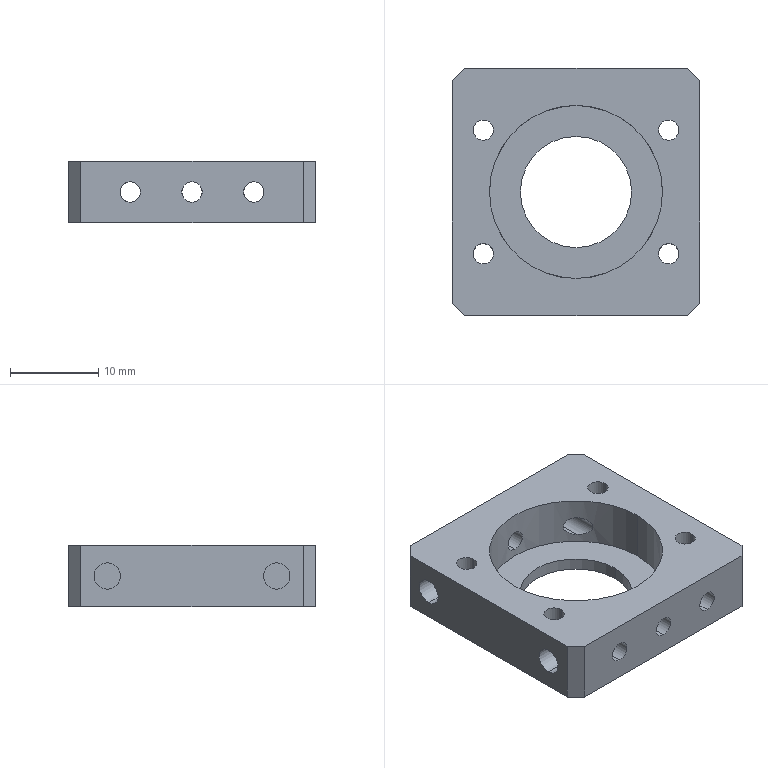Part | SolidWorks | features SplitBody 1 | 1 solid | 41 faces | box 28 x 28 x 7 mm | volume 3281 mm3 | cylinder 28 | plane 13 | commonest cylinder face diameters 2.31 x20 3 x4 12.6 x2 19.6 x2